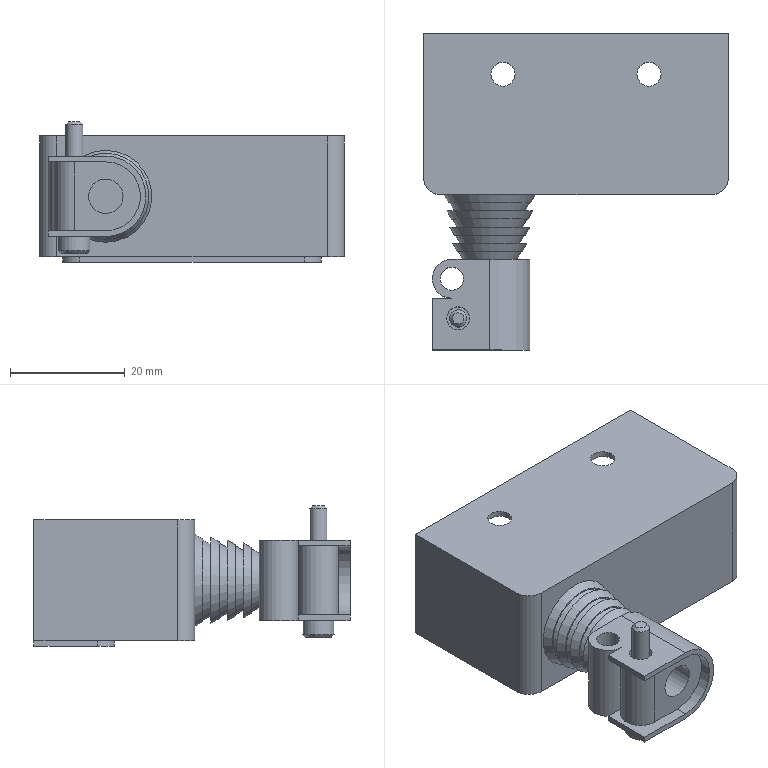Part | NX | features MFD10-WL40_1 2 | 1 solid | 212 faces | box 53 x 55 x 24.5 mm | volume 9109 mm3 | plane 160 | cylinder 42 | cone 10 | commonest cylinder face diameters 6 x5 4 x4 4.2 x4 1.1 x2 1.312 x2 1.316 x2